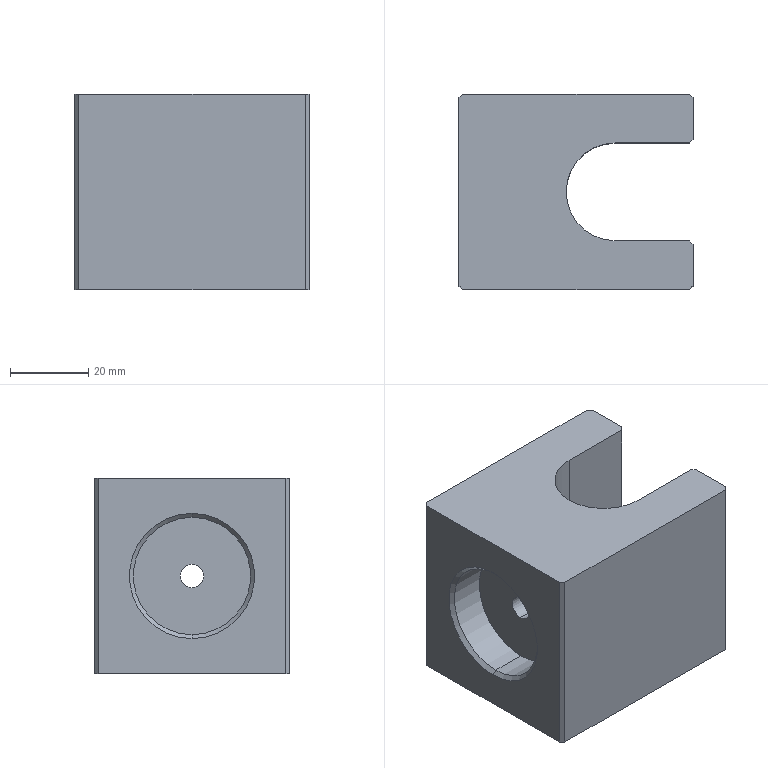Part | STEP file | Square block | 1 solid | 42 faces | box 60 x 50 x 50 mm | volume 104625 mm3 | plane 22 | cylinder 18 | cone 2 | commonest cylinder face diameters 3 x12 6 x2 25 x2 30 x2
STEP:
#1=CARTESIAN_POINT('',(-2.608,-19.158,50.));
#2=VERTEX_POINT('',#1);
#3=CARTESIAN_POINT('',(9.892,-6.658,50.));
#4=VERTEX_POINT('',#3);
#5=CARTESIAN_POINT('',(9.892,-19.158,50.));
#6=DIRECTION('',(0.,0.,-1.));
#7=DIRECTION('',(-1.,0.,0.));
#8=AXIS2_PLACEMENT_3D('',#5,#6,#7);
#9=CIRCLE('',#8,12.5);
#10=EDGE_CURVE('',#2,#4,#9,.T.);
#11=ORIENTED_EDGE('',*,*,#10,.F.);
#12=CARTESIAN_POINT('',(-2.608,-19.158,28.));
#13=VERTEX_POINT('',#12);
#14=CARTESIAN_POINT('',(-2.608,-19.158,50.));
#15=DIRECTION('',(0.,0.,-1.));
#16=VECTOR('',#15,1000.);
#17=LINE('',#14,#16);
#18=EDGE_CURVE('',#2,#13,#17,.T.);
#19=ORIENTED_EDGE('',*,*,#18,.T.);
#20=CARTESIAN_POINT('',(-2.608,-19.158,22.));
#21=VERTEX_POINT('',#20);
#22=CARTESIAN_POINT('',(-2.608,-19.158,22.));
#23=CARTESIAN_POINT('',(-2.608,-18.959,22.));
#24=CARTESIAN_POINT('',(-2.603,-18.764,22.02));
#25=CARTESIAN_POINT('',(-2.585,-18.379,22.096));
#26=CARTESIAN_POINT('',(-2.571,-18.188,22.154));
#27=CARTESIAN_POINT('',(-2.538,-17.825,22.305));
#28=CARTESIAN_POINT('',(-2.518,-17.653,22.397));
#29=CARTESIAN_POINT('',(-2.474,-17.328,22.615));
#30=CARTESIAN_POINT('',(-2.45,-17.174,22.741));
#31=CARTESIAN_POINT('',(-2.403,-16.899,23.017));
#32=CARTESIAN_POINT('',(-2.379,-16.775,23.167));
#33=CARTESIAN_POINT('',(-2.334,-16.556,23.495));
#34=CARTESIAN_POINT('',(-2.314,-16.463,23.668));
#35=CARTESIAN_POINT('',(-2.28,-16.313,24.029));
#36=CARTESIAN_POINT('',(-2.266,-16.255,24.218));
#37=CARTESIAN_POINT('',(-2.247,-16.177,24.606));
#38=CARTESIAN_POINT('',(-2.242,-16.158,24.801));
#39=CARTESIAN_POINT('',(-2.242,-16.158,25.194));
#40=CARTESIAN_POINT('',(-2.247,-16.177,25.393));
#41=CARTESIAN_POINT('',(-2.266,-16.254,25.779));
#42=CARTESIAN_POINT('',(-2.279,-16.311,25.966));
#43=CARTESIAN_POINT('',(-2.314,-16.462,26.33));
#44=CARTESIAN_POINT('',(-2.334,-16.555,26.505));
#45=CARTESIAN_POINT('',(-2.378,-16.772,26.829));
#46=CARTESIAN_POINT('',(-2.402,-16.897,26.981));
#47=CARTESIAN_POINT('',(-2.45,-17.175,27.259));
#48=CARTESIAN_POINT('',(-2.474,-17.325,27.383));
#49=CARTESIAN_POINT('',(-2.517,-17.649,27.6));
#50=CARTESIAN_POINT('',(-2.538,-17.825,27.695));
#51=CARTESIAN_POINT('',(-2.571,-18.187,27.845));
#52=CARTESIAN_POINT('',(-2.585,-18.374,27.902));
#53=CARTESIAN_POINT('',(-2.603,-18.76,27.98));
#54=CARTESIAN_POINT('',(-2.608,-18.959,28.));
#55=CARTESIAN_POINT('',(-2.608,-19.158,28.));
#56=B_SPLINE_CURVE_WITH_KNOTS('',3,(#22,#23,#24,#25,#26,#27,#28,#29,#30,#31,#32,#33,#34,#35,#36,#37,#38,#39,#40,#41,#42,#43,#44,#45,#46,#47,#48,#49,#50,#51,#52,#53,#54,#55),.UNSPECIFIED.,.F.,.F.,(4,2,2,2,2,2,2,2,2,2,2,2,2,2,2,2,4),(0.,0.0005882,0.001176,0.001765,0.002353,0.002941,0.003529,0.004117,0.004706,0.005294,0.005882,0.00647,0.007058,0.007646,0.008235,0.008823,0.009411),.UNSPECIFIED.);
#57=EDGE_CURVE('',#21,#13,#56,.T.);
#58=ORIENTED_EDGE('',*,*,#57,.F.);
#59=CARTESIAN_POINT('',(-2.608,-19.158,0.));
#60=VERTEX_POINT('',#59);
#61=CARTESIAN_POINT('',(-2.608,-19.158,50.));
#62=DIRECTION('',(0.,0.,-1.));
#63=VECTOR('',#62,1000.);
#64=LINE('',#61,#63);
#65=EDGE_CURVE('',#21,#60,#64,.T.);
#66=ORIENTED_EDGE('',*,*,#65,.T.);
#67=CARTESIAN_POINT('',(9.892,-6.658,0.));
#68=VERTEX_POINT('',#67);
#69=CARTESIAN_POINT('',(9.892,-19.158,0.));
#70=DIRECTION('',(0.,0.,-1.));
#71=DIRECTION('',(-1.,0.,0.));
#72=AXIS2_PLACEMENT_3D('',#69,#70,#71);
#73=CIRCLE('',#72,12.5);
#74=EDGE_CURVE('',#60,#68,#73,.T.);
#75=ORIENTED_EDGE('',*,*,#74,.T.);
#76=CARTESIAN_POINT('',(9.892,-6.658,50.));
#77=DIRECTION('',(0.,0.,1.));
#78=VECTOR('',#77,1000.);
#79=LINE('',#76,#78);
#80=EDGE_CURVE('',#68,#4,#79,.T.);
#81=ORIENTED_EDGE('',*,*,#80,.T.);
#82=EDGE_LOOP('',(#11,#19,#58,#66,#75,#81));
#83=FACE_OUTER_BOUND('',#82,.T.);
#84=CARTESIAN_POINT('',(9.892,-19.158,50.));
#85=DIRECTION('',(0.,0.,-1.));
#86=DIRECTION('',(-1.,0.,0.));
#87=AXIS2_PLACEMENT_3D('',#84,#85,#86);
#88=CYLINDRICAL_SURFACE('',#87,12.5);
#89=ADVANCED_FACE('',(#83),#88,.F.);
#90=CARTESIAN_POINT('',(-25.108,-2.158,24.));
#91=VERTEX_POINT('',#90);
#92=CARTESIAN_POINT('',(-25.108,-2.158,27.));
#93=VERTEX_POINT('',#92);
#94=CARTESIAN_POINT('',(-25.108,-2.158,25.5));
#95=DIRECTION('',(0.,1.,0.));
#96=DIRECTION('',(0.,0.,1.));
#97=AXIS2_PLACEMENT_3D('',#94,#95,#96);
#98=CIRCLE('',#97,1.5);
#99=EDGE_CURVE('',#91,#93,#98,.T.);
#100=ORIENTED_EDGE('',*,*,#99,.F.);
#101=CARTESIAN_POINT('',(-25.108,5.842,24.));
#102=VERTEX_POINT('',#101);
#103=CARTESIAN_POINT('',(-25.108,-2.158,24.));
#104=DIRECTION('',(0.,1.,0.));
#105=VECTOR('',#104,1000.);
#106=LINE('',#103,#105);
#107=EDGE_CURVE('',#91,#102,#106,.T.);
#108=ORIENTED_EDGE('',*,*,#107,.T.);
#109=CARTESIAN_POINT('',(-25.108,5.842,27.));
#110=VERTEX_POINT('',#109);
#111=CARTESIAN_POINT('',(-25.108,5.842,25.5));
#112=DIRECTION('',(0.,1.,0.));
#113=DIRECTION('',(0.,0.,1.));
#114=AXIS2_PLACEMENT_3D('',#111,#112,#113);
#115=CIRCLE('',#114,1.5);
#116=EDGE_CURVE('',#102,#110,#115,.T.);
#117=ORIENTED_EDGE('',*,*,#116,.T.);
#118=CARTESIAN_POINT('',(-25.108,-2.158,27.));
#119=DIRECTION('',(0.,1.,0.));
#120=VECTOR('',#119,1000.);
#121=LINE('',#118,#120);
#122=EDGE_CURVE('',#93,#110,#121,.T.);
#123=ORIENTED_EDGE('',*,*,#122,.F.);
#124=EDGE_LOOP('',(#100,#108,#117,#123));
#125=FACE_OUTER_BOUND('',#124,.T.);
#126=CARTESIAN_POINT('',(-25.108,-2.158,25.5));
#127=DIRECTION('',(0.,1.,0.));
#128=DIRECTION('',(0.,0.,1.));
#129=AXIS2_PLACEMENT_3D('',#126,#127,#128);
#130=CYLINDRICAL_SURFACE('',#129,1.5);
#131=ADVANCED_FACE('',(#125),#130,.F.);
#132=CARTESIAN_POINT('',(-15.108,-2.158,24.));
#133=VERTEX_POINT('',#132);
#134=CARTESIAN_POINT('',(-15.108,-2.158,27.));
#135=VERTEX_POINT('',#134);
#136=CARTESIAN_POINT('',(-15.108,-2.158,25.5));
#137=DIRECTION('',(0.,1.,0.));
#138=DIRECTION('',(0.,0.,1.));
#139=AXIS2_PLACEMENT_3D('',#136,#137,#138);
#140=CIRCLE('',#139,1.5);
#141=EDGE_CURVE('',#133,#135,#140,.T.);
#142=ORIENTED_EDGE('',*,*,#141,.F.);
#143=CARTESIAN_POINT('',(-15.108,5.842,24.));
#144=VERTEX_POINT('',#143);
#145=CARTESIAN_POINT('',(-15.108,-2.158,24.));
#146=DIRECTION('',(0.,1.,0.));
#147=VECTOR('',#146,1000.);
#148=LINE('',#145,#147);
#149=EDGE_CURVE('',#133,#144,#148,.T.);
#150=ORIENTED_EDGE('',*,*,#149,.T.);
#151=CARTESIAN_POINT('',(-15.108,5.842,27.));
#152=VERTEX_POINT('',#151);
#153=CARTESIAN_POINT('',(-15.108,5.842,25.5));
#154=DIRECTION('',(0.,1.,0.));
#155=DIRECTION('',(0.,0.,1.));
#156=AXIS2_PLACEMENT_3D('',#153,#154,#155);
#157=CIRCLE('',#156,1.5);
#158=EDGE_CURVE('',#144,#152,#157,.T.);
#159=ORIENTED_EDGE('',*,*,#158,.T.);
#160=CARTESIAN_POINT('',(-15.108,-2.158,27.));
#161=DIRECTION('',(0.,1.,0.));
#162=VECTOR('',#161,1000.);
#163=LINE('',#160,#162);
#164=EDGE_CURVE('',#135,#152,#163,.T.);
#165=ORIENTED_EDGE('',*,*,#164,.F.);
#166=EDGE_LOOP('',(#142,#150,#159,#165));
#167=FACE_OUTER_BOUND('',#166,.T.);
#168=CARTESIAN_POINT('',(-15.108,-2.158,25.5));
#169=DIRECTION('',(0.,1.,0.));
#170=DIRECTION('',(0.,0.,1.));
#171=AXIS2_PLACEMENT_3D('',#168,#169,#170);
#172=CYLINDRICAL_SURFACE('',#171,1.5);
#173=ADVANCED_FACE('',(#167),#172,.F.);
#174=CARTESIAN_POINT('',(-25.108,-2.158,39.));
#175=VERTEX_POINT('',#174);
#176=CARTESIAN_POINT('',(-25.108,-2.158,42.));
#177=VERTEX_POINT('',#176);
#178=CARTESIAN_POINT('',(-25.108,-2.158,40.5));
#179=DIRECTION('',(0.,1.,0.));
#180=DIRECTION('',(0.,0.,1.));
#181=AXIS2_PLACEMENT_3D('',#178,#179,#180);
#182=CIRCLE('',#181,1.5);
#183=EDGE_CURVE('',#175,#177,#182,.T.);
#184=ORIENTED_EDGE('',*,*,#183,.F.);
#185=CARTESIAN_POINT('',(-25.108,5.842,39.));
#186=VERTEX_POINT('',#185);
#187=CARTESIAN_POINT('',(-25.108,-2.158,39.));
#188=DIRECTION('',(0.,1.,0.));
#189=VECTOR('',#188,1000.);
#190=LINE('',#187,#189);
#191=EDGE_CURVE('',#175,#186,#190,.T.);
#192=ORIENTED_EDGE('',*,*,#191,.T.);
#193=CARTESIAN_POINT('',(-25.108,5.842,42.));
#194=VERTEX_POINT('',#193);
#195=CARTESIAN_POINT('',(-25.108,5.842,40.5));
#196=DIRECTION('',(0.,1.,0.));
#197=DIRECTION('',(0.,0.,1.));
#198=AXIS2_PLACEMENT_3D('',#195,#196,#197);
#199=CIRCLE('',#198,1.5);
#200=EDGE_CURVE('',#186,#194,#199,.T.);
#201=ORIENTED_EDGE('',*,*,#200,.T.);
#202=CARTESIAN_POINT('',(-25.108,-2.158,42.));
#203=DIRECTION('',(0.,1.,0.));
#204=VECTOR('',#203,1000.);
#205=LINE('',#202,#204);
#206=EDGE_CURVE('',#177,#194,#205,.T.);
#207=ORIENTED_EDGE('',*,*,#206,.F.);
#208=EDGE_LOOP('',(#184,#192,#201,#207));
#209=FACE_OUTER_BOUND('',#208,.T.);
#210=CARTESIAN_POINT('',(-25.108,-2.158,40.5));
#211=DIRECTION('',(0.,1.,0.));
#212=DIRECTION('',(0.,0.,1.));
#213=AXIS2_PLACEMENT_3D('',#210,#211,#212);
#214=CYLINDRICAL_SURFACE('',#213,1.5);
#215=ADVANCED_FACE('',(#209),#214,.F.);
#216=CARTESIAN_POINT('',(-15.108,-2.158,39.));
#217=VERTEX_POINT('',#216);
#218=CARTESIAN_POINT('',(-15.108,-2.158,42.));
#219=VERTEX_POINT('',#218);
#220=CARTESIAN_POINT('',(-15.108,-2.158,40.5));
#221=DIRECTION('',(0.,1.,0.));
#222=DIRECTION('',(0.,0.,1.));
#223=AXIS2_PLACEMENT_3D('',#220,#221,#222);
#224=CIRCLE('',#223,1.5);
#225=EDGE_CURVE('',#217,#219,#224,.T.);
#226=ORIENTED_EDGE('',*,*,#225,.F.);
#227=CARTESIAN_POINT('',(-15.108,5.842,39.));
#228=VERTEX_POINT('',#227);
#229=CARTESIAN_POINT('',(-15.108,-2.158,39.));
#230=DIRECTION('',(0.,1.,0.));
#231=VECTOR('',#230,1000.);
#232=LINE('',#229,#231);
#233=EDGE_CURVE('',#217,#228,#232,.T.);
#234=ORIENTED_EDGE('',*,*,#233,.T.);
#235=CARTESIAN_POINT('',(-15.108,5.842,42.));
#236=VERTEX_POINT('',#235);
#237=CARTESIAN_POINT('',(-15.108,5.842,40.5));
#238=DIRECTION('',(0.,1.,0.));
#239=DIRECTION('',(0.,0.,1.));
#240=AXIS2_PLACEMENT_3D('',#237,#238,#239);
#241=CIRCLE('',#240,1.5);
#242=EDGE_CURVE('',#228,#236,#241,.T.);
#243=ORIENTED_EDGE('',*,*,#242,.T.);
#244=CARTESIAN_POINT('',(-15.108,-2.158,42.));
#245=DIRECTION('',(0.,1.,0.));
#246=VECTOR('',#245,1000.);
#247=LINE('',#244,#246);
#248=EDGE_CURVE('',#219,#236,#247,.T.);
#249=ORIENTED_EDGE('',*,*,#248,.F.);
#250=EDGE_LOOP('',(#226,#234,#243,#249));
#251=FACE_OUTER_BOUND('',#250,.T.);
#252=CARTESIAN_POINT('',(-15.108,-2.158,40.5));
#253=DIRECTION('',(0.,1.,0.));
#254=DIRECTION('',(0.,0.,1.));
#255=AXIS2_PLACEMENT_3D('',#252,#253,#254);
#256=CYLINDRICAL_SURFACE('',#255,1.5);
#257=ADVANCED_FACE('',(#251),#256,.F.);
#258=CARTESIAN_POINT('',(-15.108,-2.158,9.));
#259=VERTEX_POINT('',#258);
#260=CARTESIAN_POINT('',(-15.108,-2.158,12.));
#261=VERTEX_POINT('',#260);
#262=CARTESIAN_POINT('',(-15.108,-2.158,10.5));
#263=DIRECTION('',(0.,1.,0.));
#264=DIRECTION('',(0.,0.,1.));
#265=AXIS2_PLACEMENT_3D('',#262,#263,#264);
#266=CIRCLE('',#265,1.5);
#267=EDGE_CURVE('',#259,#261,#266,.T.);
#268=ORIENTED_EDGE('',*,*,#267,.F.);
#269=CARTESIAN_POINT('',(-15.108,5.842,9.));
#270=VERTEX_POINT('',#269);
#271=CARTESIAN_POINT('',(-15.108,-2.158,9.));
#272=DIRECTION('',(0.,1.,0.));
#273=VECTOR('',#272,1000.);
#274=LINE('',#271,#273);
#275=EDGE_CURVE('',#259,#270,#274,.T.);
#276=ORIENTED_EDGE('',*,*,#275,.T.);
#277=CARTESIAN_POINT('',(-15.108,5.842,12.));
#278=VERTEX_POINT('',#277);
#279=CARTESIAN_POINT('',(-15.108,5.842,10.5));
#280=DIRECTION('',(0.,1.,0.));
#281=DIRECTION('',(0.,0.,1.));
#282=AXIS2_PLACEMENT_3D('',#279,#280,#281);
#283=CIRCLE('',#282,1.5);
#284=EDGE_CURVE('',#270,#278,#283,.T.);
#285=ORIENTED_EDGE('',*,*,#284,.T.);
#286=CARTESIAN_POINT('',(-15.108,-2.158,12.));
#287=DIRECTION('',(0.,1.,0.));
#288=VECTOR('',#287,1000.);
#289=LINE('',#286,#288);
#290=EDGE_CURVE('',#261,#278,#289,.T.);
#291=ORIENTED_EDGE('',*,*,#290,.F.);
#292=EDGE_LOOP('',(#268,#276,#285,#291));
#293=FACE_OUTER_BOUND('',#292,.T.);
#294=CARTESIAN_POINT('',(-15.108,-2.158,10.5));
#295=DIRECTION('',(0.,1.,0.));
#296=DIRECTION('',(0.,0.,1.));
#297=AXIS2_PLACEMENT_3D('',#294,#295,#296);
#298=CYLINDRICAL_SURFACE('',#297,1.5);
#299=ADVANCED_FACE('',(#293),#298,.F.);
#300=CARTESIAN_POINT('',(-25.108,-2.158,9.));
#301=VERTEX_POINT('',#300);
#302=CARTESIAN_POINT('',(-25.108,-2.158,12.));
#303=VERTEX_POINT('',#302);
#304=CARTESIAN_POINT('',(-25.108,-2.158,10.5));
#305=DIRECTION('',(0.,1.,0.));
#306=DIRECTION('',(0.,0.,1.));
#307=AXIS2_PLACEMENT_3D('',#304,#305,#306);
#308=CIRCLE('',#307,1.5);
#309=EDGE_CURVE('',#301,#303,#308,.T.);
#310=ORIENTED_EDGE('',*,*,#309,.F.);
#311=CARTESIAN_POINT('',(-25.108,5.842,9.));
#312=VERTEX_POINT('',#311);
#313=CARTESIAN_POINT('',(-25.108,-2.158,9.));
#314=DIRECTION('',(0.,1.,0.));
#315=VECTOR('',#314,1000.);
#316=LINE('',#313,#315);
#317=EDGE_CURVE('',#301,#312,#316,.T.);
#318=ORIENTED_EDGE('',*,*,#317,.T.);
#319=CARTESIAN_POINT('',(-25.108,5.842,12.));
#320=VERTEX_POINT('',#319);
#321=CARTESIAN_POINT('',(-25.108,5.842,10.5));
#322=DIRECTION('',(0.,1.,0.));
#323=DIRECTION('',(0.,0.,1.));
#324=AXIS2_PLACEMENT_3D('',#321,#322,#323);
#325=CIRCLE('',#324,1.5);
#326=EDGE_CURVE('',#312,#320,#325,.T.);
#327=ORIENTED_EDGE('',*,*,#326,.T.);
#328=CARTESIAN_POINT('',(-25.108,-2.158,12.));
#329=DIRECTION('',(0.,1.,0.));
#330=VECTOR('',#329,1000.);
#331=LINE('',#328,#330);
#332=EDGE_CURVE('',#303,#320,#331,.T.);
#333=ORIENTED_EDGE('',*,*,#332,.F.);
#334=EDGE_LOOP('',(#310,#318,#327,#333));
#335=FACE_OUTER_BOUND('',#334,.T.);
#336=CARTESIAN_POINT('',(-25.108,-2.158,10.5));
#337=DIRECTION('',(0.,1.,0.));
#338=DIRECTION('',(0.,0.,1.));
#339=AXIS2_PLACEMENT_3D('',#336,#337,#338);
#340=CYLINDRICAL_SURFACE('',#339,1.5);
#341=ADVANCED_FACE('',(#335),#340,.F.);
#342=CARTESIAN_POINT('',(-2.608,-19.158,28.));
#343=CARTESIAN_POINT('',(-2.608,-19.357,28.));
#344=CARTESIAN_POINT('',(-2.603,-19.552,27.98));
#345=CARTESIAN_POINT('',(-2.585,-19.937,27.904));
#346=CARTESIAN_POINT('',(-2.571,-20.128,27.846));
#347=CARTESIAN_POINT('',(-2.538,-20.491,27.695));
#348=CARTESIAN_POINT('',(-2.518,-20.663,27.603));
#349=CARTESIAN_POINT('',(-2.474,-20.988,27.385));
#350=CARTESIAN_POINT('',(-2.45,-21.142,27.259));
#351=CARTESIAN_POINT('',(-2.403,-21.417,26.983));
#352=CARTESIAN_POINT('',(-2.379,-21.541,26.833));
#353=CARTESIAN_POINT('',(-2.334,-21.761,26.505));
#354=CARTESIAN_POINT('',(-2.314,-21.853,26.332));
#355=CARTESIAN_POINT('',(-2.28,-22.003,25.971));
#356=CARTESIAN_POINT('',(-2.266,-22.061,25.782));
#357=CARTESIAN_POINT('',(-2.247,-22.139,25.394));
#358=CARTESIAN_POINT('',(-2.242,-22.158,25.199));
#359=CARTESIAN_POINT('',(-2.242,-22.158,24.806));
#360=CARTESIAN_POINT('',(-2.247,-22.139,24.607));
#361=CARTESIAN_POINT('',(-2.266,-22.062,24.221));
#362=CARTESIAN_POINT('',(-2.279,-22.005,24.034));
#363=CARTESIAN_POINT('',(-2.314,-21.854,23.67));
#364=CARTESIAN_POINT('',(-2.334,-21.761,23.495));
#365=CARTESIAN_POINT('',(-2.378,-21.544,23.171));
#366=CARTESIAN_POINT('',(-2.402,-21.419,23.019));
#367=CARTESIAN_POINT('',(-2.45,-21.141,22.741));
#368=CARTESIAN_POINT('',(-2.474,-20.991,22.617));
#369=CARTESIAN_POINT('',(-2.517,-20.667,22.4));
#370=CARTESIAN_POINT('',(-2.538,-20.491,22.305));
#371=CARTESIAN_POINT('',(-2.571,-20.129,22.155));
#372=CARTESIAN_POINT('',(-2.585,-19.942,22.098));
#373=CARTESIAN_POINT('',(-2.603,-19.556,22.02));
#374=CARTESIAN_POINT('',(-2.608,-19.357,22.));
#375=CARTESIAN_POINT('',(-2.608,-19.158,22.));
#376=B_SPLINE_CURVE_WITH_KNOTS('',3,(#342,#343,#344,#345,#346,#347,#348,#349,#350,#351,#352,#353,#354,#355,#356,#357,#358,#359,#360,#361,#362,#363,#364,#365,#366,#367,#368,#369,#370,#371,#372,#373,#374,#375),.UNSPECIFIED.,.F.,.F.,(4,2,2,2,2,2,2,2,2,2,2,2,2,2,2,2,4),(0.009411,0.009999,0.01059,0.01118,0.01176,0.01235,0.01294,0.01353,0.01412,0.0147,0.01529,0.01588,0.01647,0.01706,0.01765,0.01823,0.01882),.UNSPECIFIED.);
#377=EDGE_CURVE('',#13,#21,#376,.T.);
#378=ORIENTED_EDGE('',*,*,#377,.T.);
#379=CARTESIAN_POINT('',(-20.108,-19.158,22.));
#380=VERTEX_POINT('',#379);
#381=CARTESIAN_POINT('',(29.892,-19.158,22.));
#382=DIRECTION('',(-1.,0.,0.));
#383=VECTOR('',#382,1000.);
#384=LINE('',#381,#383);
#385=EDGE_CURVE('',#21,#380,#384,.T.);
#386=ORIENTED_EDGE('',*,*,#385,.T.);
#387=CARTESIAN_POINT('',(-20.108,-19.158,28.));
#388=VERTEX_POINT('',#387);
#389=CARTESIAN_POINT('',(-20.108,-19.158,25.));
#390=DIRECTION('',(1.,0.,0.));
#391=DIRECTION('',(0.,0.,1.));
#392=AXIS2_PLACEMENT_3D('',#389,#390,#391);
#393=CIRCLE('',#392,3.);
#394=EDGE_CURVE('',#388,#380,#393,.T.);
#395=ORIENTED_EDGE('',*,*,#394,.F.);
#396=CARTESIAN_POINT('',(29.892,-19.158,28.));
#397=DIRECTION('',(-1.,0.,0.));
#398=VECTOR('',#397,1000.);
#399=LINE('',#396,#398);
#400=EDGE_CURVE('',#13,#388,#399,.T.);
#401=ORIENTED_EDGE('',*,*,#400,.F.);
#402=EDGE_LOOP('',(#378,#386,#395,#401));
#403=FACE_OUTER_BOUND('',#402,.T.);
#404=CARTESIAN_POINT('',(29.892,-19.158,25.));
#405=DIRECTION('',(-1.,0.,0.));
#406=DIRECTION('',(0.,0.,1.));
#407=AXIS2_PLACEMENT_3D('',#404,#405,#406);
#408=CYLINDRICAL_SURFACE('',#407,3.);
#409=ADVANCED_FACE('',(#403),#408,.F.);
#410=CARTESIAN_POINT('',(-29.108,-19.158,10.));
#411=VERTEX_POINT('',#410);
#412=CARTESIAN_POINT('',(-29.108,-19.158,40.));
#413=VERTEX_POINT('',#412);
#414=CARTESIAN_POINT('',(-29.108,-19.158,25.));
#415=DIRECTION('',(-1.,0.,0.));
#416=DIRECTION('',(0.,0.,1.));
#417=AXIS2_PLACEMENT_3D('',#414,#415,#416);
#418=CIRCLE('',#417,15.);
#419=EDGE_CURVE('',#411,#413,#418,.T.);
#420=ORIENTED_EDGE('',*,*,#419,.F.);
#421=CARTESIAN_POINT('',(-30.108,-19.158,9.));
#422=VERTEX_POINT('',#421);
#423=CARTESIAN_POINT('',(-30.108,-19.158,9.));
#424=DIRECTION('',(-0.7071,0.,-0.7071));
#425=VECTOR('',#424,1000.);
#426=LINE('',#423,#425);
#427=EDGE_CURVE('',#411,#422,#426,.T.);
#428=ORIENTED_EDGE('',*,*,#427,.T.);
#429=CARTESIAN_POINT('',(-30.108,-19.158,41.));
#430=VERTEX_POINT('',#429);
#431=CARTESIAN_POINT('',(-30.108,-19.158,25.));
#432=DIRECTION('',(-1.,0.,0.));
#433=DIRECTION('',(0.,0.,1.));
#434=AXIS2_PLACEMENT_3D('',#431,#432,#433);
#435=CIRCLE('',#434,16.);
#436=EDGE_CURVE('',#422,#430,#435,.T.);
#437=ORIENTED_EDGE('',*,*,#436,.T.);
#438=CARTESIAN_POINT('',(-30.108,-19.158,41.));
#439=DIRECTION('',(-0.7071,0.,0.7071));
#440=VECTOR('',#439,1000.);
#441=LINE('',#438,#440);
#442=EDGE_CURVE('',#413,#430,#441,.T.);
#443=ORIENTED_EDGE('',*,*,#442,.F.);
#444=EDGE_LOOP('',(#420,#428,#437,#443));
#445=FACE_OUTER_BOUND('',#444,.T.);
#446=CARTESIAN_POINT('',(-30.108,-19.158,25.));
#447=DIRECTION('',(-1.,0.,0.));
#448=DIRECTION('',(0.,0.,1.));
#449=AXIS2_PLACEMENT_3D('',#446,#447,#448);
#450=CONICAL_SURFACE('',#449,16.,0.7854);
#451=ADVANCED_FACE('',(#445),#450,.F.);
#452=CARTESIAN_POINT('',(-20.108,-19.158,10.));
#453=VERTEX_POINT('',#452);
#454=CARTESIAN_POINT('',(-20.108,-19.158,40.));
#455=VERTEX_POINT('',#454);
#456=CARTESIAN_POINT('',(-20.108,-19.158,25.));
#457=DIRECTION('',(-1.,0.,0.));
#458=DIRECTION('',(0.,0.,1.));
#459=AXIS2_PLACEMENT_3D('',#456,#457,#458);
#460=CIRCLE('',#459,15.);
#461=EDGE_CURVE('',#453,#455,#460,.T.);
#462=ORIENTED_EDGE('',*,*,#461,.F.);
#463=CARTESIAN_POINT('',(-20.108,-19.158,10.));
#464=DIRECTION('',(-1.,0.,0.));
#465=VECTOR('',#464,1000.);
#466=LINE('',#463,#465);
#467=EDGE_CURVE('',#453,#411,#466,.T.);
#468=ORIENTED_EDGE('',*,*,#467,.T.);
#469=ORIENTED_EDGE('',*,*,#419,.T.);
#470=CARTESIAN_POINT('',(-20.108,-19.158,40.));
#471=DIRECTION('',(-1.,0.,0.));
#472=VECTOR('',#471,1000.);
#473=LINE('',#470,#472);
#474=EDGE_CURVE('',#455,#413,#473,.T.);
#475=ORIENTED_EDGE('',*,*,#474,.F.);
#476=EDGE_LOOP('',(#462,#468,#469,#475));
#477=FACE_OUTER_BOUND('',#476,.T.);
#478=CARTESIAN_POINT('',(-20.108,-19.158,25.));
#479=DIRECTION('',(-1.,0.,0.));
#480=DIRECTION('',(0.,0.,1.));
#481=AXIS2_PLACEMENT_3D('',#478,#479,#480);
#482=CYLINDRICAL_SURFACE('',#481,15.);
#483=ADVANCED_FACE('',(#477),#482,.F.);
#484=CARTESIAN_POINT('',(-29.108,-44.158,0.));
#485=VERTEX_POINT('',#484);
#486=CARTESIAN_POINT('',(-29.108,-44.158,50.));
#487=VERTEX_POINT('',#486);
#488=CARTESIAN_POINT('',(-29.108,-44.158,50.));
#489=DIRECTION('',(0.,0.,1.));
#490=VECTOR('',#489,1000.);
#491=LINE('',#488,#490);
#492=EDGE_CURVE('',#485,#487,#491,.T.);
#493=ORIENTED_EDGE('',*,*,#492,.F.);
#494=CARTESIAN_POINT('',(28.892,-44.158,0.));
#495=VERTEX_POINT('',#494);
#496=CARTESIAN_POINT('',(-30.108,-44.158,0.));
#497=DIRECTION('',(-1.,0.,0.));
#498=VECTOR('',#497,1000.);
#499=LINE('',#496,#498);
#500=EDGE_CURVE('',#495,#485,#499,.T.);
#501=ORIENTED_EDGE('',*,*,#500,.F.);
#502=CARTESIAN_POINT('',(28.892,-44.158,50.));
#503=VERTEX_POINT('',#502);
#504=CARTESIAN_POINT('',(28.892,-44.158,50.));
#505=DIRECTION('',(0.,0.,-1.));
#506=VECTOR('',#505,1000.);
#507=LINE('',#504,#506);
#508=EDGE_CURVE('',#503,#495,#507,.T.);
#509=ORIENTED_EDGE('',*,*,#508,.F.);
#510=CARTESIAN_POINT('',(-30.108,-44.158,50.));
#511=DIRECTION('',(1.,0.,0.));
#512=VECTOR('',#511,1000.);
#513=LINE('',#510,#512);
#514=EDGE_CURVE('',#487,#503,#513,.T.);
#515=ORIENTED_EDGE('',*,*,#514,.F.);
#516=EDGE_LOOP('',(#493,#501,#509,#515));
#517=FACE_OUTER_BOUND('',#516,.T.);
#518=CARTESIAN_POINT('',(-30.108,-44.158,50.));
#519=DIRECTION('',(0.,1.,0.));
#520=DIRECTION('',(0.,0.,1.));
#521=AXIS2_PLACEMENT_3D('',#518,#519,#520);
#522=PLANE('',#521);
#523=ADVANCED_FACE('',(#517),#522,.F.);
#524=CARTESIAN_POINT('',(28.892,5.842,50.));
#525=VERTEX_POINT('',#524);
#526=CARTESIAN_POINT('',(-29.108,5.842,50.));
#527=VERTEX_POINT('',#526);
#528=CARTESIAN_POINT('',(9.892,5.842,50.));
#529=DIRECTION('',(-1.,0.,0.));
#530=VECTOR('',#529,1000.);
#531=LINE('',#528,#530);
#532=EDGE_CURVE('',#525,#527,#531,.T.);
#533=ORIENTED_EDGE('',*,*,#532,.T.);
#534=CARTESIAN_POINT('',(-30.108,4.842,50.));
#535=VERTEX_POINT('',#534);
#536=CARTESIAN_POINT('',(-30.108,4.842,50.));
#537=DIRECTION('',(-0.7071,-0.7071,0.));
#538=VECTOR('',#537,1000.);
#539=LINE('',#536,#538);
#540=EDGE_CURVE('',#527,#535,#539,.T.);
#541=ORIENTED_EDGE('',*,*,#540,.T.);
#542=CARTESIAN_POINT('',(-30.108,-43.158,50.));
#543=VERTEX_POINT('',#542);
#544=CARTESIAN_POINT('',(-30.108,-19.158,50.));
#545=DIRECTION('',(0.,-1.,0.));
#546=VECTOR('',#545,1000.);
#547=LINE('',#544,#546);
#548=EDGE_CURVE('',#535,#543,#547,.T.);
#549=ORIENTED_EDGE('',*,*,#548,.T.);
#550=CARTESIAN_POINT('',(-30.108,-43.158,50.));
#551=DIRECTION('',(0.7071,-0.7071,0.));
#552=VECTOR('',#551,1000.);
#553=LINE('',#550,#552);
#554=EDGE_CURVE('',#543,#487,#553,.T.);
#555=ORIENTED_EDGE('',*,*,#554,.T.);
#556=ORIENTED_EDGE('',*,*,#514,.T.);
#557=CARTESIAN_POINT('',(29.892,-43.158,50.));
#558=VERTEX_POINT('',#557);
#559=CARTESIAN_POINT('',(28.892,-44.158,50.));
#560=DIRECTION('',(0.7071,0.7071,0.));
#561=VECTOR('',#560,1000.);
#562=LINE('',#559,#561);
#563=EDGE_CURVE('',#503,#558,#562,.T.);
#564=ORIENTED_EDGE('',*,*,#563,.T.);
#565=CARTESIAN_POINT('',(29.892,-32.658,50.));
#566=VERTEX_POINT('',#565);
#567=CARTESIAN_POINT('',(29.892,-19.158,50.));
#568=DIRECTION('',(0.,1.,0.));
#569=VECTOR('',#568,1000.);
#570=LINE('',#567,#569);
#571=EDGE_CURVE('',#558,#566,#570,.T.);
#572=ORIENTED_EDGE('',*,*,#571,.T.);
#573=CARTESIAN_POINT('',(28.892,-31.658,50.));
#574=VERTEX_POINT('',#573);
#575=CARTESIAN_POINT('',(28.892,-31.658,50.));
#576=DIRECTION('',(-0.7071,0.7071,0.));
#577=VECTOR('',#576,1000.);
#578=LINE('',#575,#577);
#579=EDGE_CURVE('',#566,#574,#578,.T.);
#580=ORIENTED_EDGE('',*,*,#579,.T.);
#581=CARTESIAN_POINT('',(9.892,-31.658,50.));
#582=VERTEX_POINT('',#581);
#583=CARTESIAN_POINT('',(9.892,-31.658,50.));
#584=DIRECTION('',(-1.,0.,0.));
#585=VECTOR('',#584,1000.);
#586=LINE('',#583,#585);
#587=EDGE_CURVE('',#574,#582,#586,.T.);
#588=ORIENTED_EDGE('',*,*,#587,.T.);
#589=CARTESIAN_POINT('',(9.892,-19.158,50.));
#590=DIRECTION('',(0.,0.,-1.));
#591=DIRECTION('',(-1.,0.,0.));
#592=AXIS2_PLACEMENT_3D('',#589,#590,#591);
#593=CIRCLE('',#592,12.5);
#594=EDGE_CURVE('',#582,#2,#593,.T.);
#595=ORIENTED_EDGE('',*,*,#594,.T.);
#596=ORIENTED_EDGE('',*,*,#10,.T.);
#597=CARTESIAN_POINT('',(28.892,-6.658,50.));
#598=VERTEX_POINT('',#597);
#599=CARTESIAN_POINT('',(9.892,-6.658,50.));
#600=DIRECTION('',(1.,0.,0.));
#601=VECTOR('',#600,1000.);
#602=LINE('',#599,#601);
#603=EDGE_CURVE('',#4,#598,#602,.T.);
#604=ORIENTED_EDGE('',*,*,#603,.T.);
#605=CARTESIAN_POINT('',(29.892,-5.658,50.));
#606=VERTEX_POINT('',#605);
#607=CARTESIAN_POINT('',(29.892,-5.658,50.));
#608=DIRECTION('',(0.7071,0.7071,0.));
#609=VECTOR('',#608,1000.);
#610=LINE('',#607,#609);
#611=EDGE_CURVE('',#598,#606,#610,.T.);
#612=ORIENTED_EDGE('',*,*,#611,.T.);
#613=CARTESIAN_POINT('',(29.892,4.842,50.));
#614=VERTEX_POINT('',#613);
#615=CARTESIAN_POINT('',(29.892,-19.158,50.));
#616=DIRECTION('',(0.,1.,0.));
#617=VECTOR('',#616,1000.);
#618=LINE('',#615,#617);
#619=EDGE_CURVE('',#606,#614,#618,.T.);
#620=ORIENTED_EDGE('',*,*,#619,.T.);
#621=CARTESIAN_POINT('',(28.892,5.842,50.));
#622=DIRECTION('',(-0.7071,0.7071,0.));
#623=VECTOR('',#622,1000.);
#624=LINE('',#621,#623);
#625=EDGE_CURVE('',#614,#525,#624,.T.);
#626=ORIENTED_EDGE('',*,*,#625,.T.);
#627=EDGE_LOOP('',(#533,#541,#549,#555,#556,#564,#572,#580,#588,#595,#596,#604,#612,#620,#626));
#628=FACE_OUTER_BOUND('',#627,.T.);
#629=CARTESIAN_POINT('',(9.892,-19.158,50.));
#630=DIRECTION('',(0.,0.,1.));
#631=DIRECTION('',(1.,0.,0.));
#632=AXIS2_PLACEMENT_3D('',#629,#630,#631);
#633=PLANE('',#632);
#634=ADVANCED_FACE('',(#628),#633,.T.);
#635=CARTESIAN_POINT('',(-30.108,-43.158,0.));
#636=VERTEX_POINT('',#635);
#637=CARTESIAN_POINT('',(-30.108,-43.158,50.));
#638=DIRECTION('',(0.,0.,1.));
#639=VECTOR('',#638,1000.);
#640=LINE('',#637,#639);
#641=EDGE_CURVE('',#636,#543,#640,.T.);
#642=ORIENTED_EDGE('',*,*,#641,.F.);
#643=CARTESIAN_POINT('',(-29.108,-44.158,0.));
#644=DIRECTION('',(-0.7071,0.7071,0.));
#645=VECTOR('',#644,1000.);
#646=LINE('',#643,#645);
#647=EDGE_CURVE('',#485,#636,#646,.T.);
#648=ORIENTED_EDGE('',*,*,#647,.F.);
#649=ORIENTED_EDGE('',*,*,#492,.T.);
#650=ORIENTED_EDGE('',*,*,#554,.F.);
#651=EDGE_LOOP('',(#642,#648,#649,#650));
#652=FACE_OUTER_BOUND('',#651,.T.);
#653=CARTESIAN_POINT('',(-29.108,-44.158,50.));
#654=DIRECTION('',(0.7071,0.7071,0.));
#655=DIRECTION('',(-0.7071,0.7071,0.));
#656=AXIS2_PLACEMENT_3D('',#653,#654,#655);
#657=PLANE('',#656);
#658=ADVANCED_FACE('',(#652),#657,.F.);
#659=ORIENTED_EDGE('',*,*,#647,.T.);
#660=CARTESIAN_POINT('',(-30.108,4.842,0.));
#661=VERTEX_POINT('',#660);
#662=CARTESIAN_POINT('',(-30.108,-19.158,0.));
#663=DIRECTION('',(0.,-1.,0.));
#664=VECTOR('',#663,1000.);
#665=LINE('',#662,#664);
#666=EDGE_CURVE('',#661,#636,#665,.T.);
#667=ORIENTED_EDGE('',*,*,#666,.F.);
#668=CARTESIAN_POINT('',(-29.108,5.842,0.));
#669=VERTEX_POINT('',#668);
#670=CARTESIAN_POINT('',(-30.108,4.842,0.));
#671=DIRECTION('',(0.7071,0.7071,0.));
#672=VECTOR('',#671,1000.);
#673=LINE('',#670,#672);
#674=EDGE_CURVE('',#661,#669,#673,.T.);
#675=ORIENTED_EDGE('',*,*,#674,.T.);
#676=CARTESIAN_POINT('',(28.892,5.842,0.));
#677=VERTEX_POINT('',#676);
#678=CARTESIAN_POINT('',(9.892,5.842,0.));
#679=DIRECTION('',(-1.,0.,0.));
#680=VECTOR('',#679,1000.);
#681=LINE('',#678,#680);
#682=EDGE_CURVE('',#677,#669,#681,.T.);
#683=ORIENTED_EDGE('',*,*,#682,.F.);
#684=CARTESIAN_POINT('',(29.892,4.842,0.));
#685=VERTEX_POINT('',#684);
#686=CARTESIAN_POINT('',(28.892,5.842,0.));
#687=DIRECTION('',(0.7071,-0.7071,0.));
#688=VECTOR('',#687,1000.);
#689=LINE('',#686,#688);
#690=EDGE_CURVE('',#677,#685,#689,.T.);
#691=ORIENTED_EDGE('',*,*,#690,.T.);
#692=CARTESIAN_POINT('',(29.892,-5.658,0.));
#693=VERTEX_POINT('',#692);
#694=CARTESIAN_POINT('',(29.892,-19.158,0.));
#695=DIRECTION('',(0.,1.,0.));
#696=VECTOR('',#695,1000.);
#697=LINE('',#694,#696);
#698=EDGE_CURVE('',#693,#685,#697,.T.);
#699=ORIENTED_EDGE('',*,*,#698,.F.);
#700=CARTESIAN_POINT('',(28.892,-6.658,0.));
#701=VERTEX_POINT('',#700);
#702=CARTESIAN_POINT('',(29.892,-5.658,0.));
#703=DIRECTION('',(-0.7071,-0.7071,0.));
#704=VECTOR('',#703,1000.);
#705=LINE('',#702,#704);
#706=EDGE_CURVE('',#693,#701,#705,.T.);
#707=ORIENTED_EDGE('',*,*,#706,.T.);
#708=CARTESIAN_POINT('',(9.892,-6.658,0.));
#709=DIRECTION('',(1.,0.,0.));
#710=VECTOR('',#709,1000.);
#711=LINE('',#708,#710);
#712=EDGE_CURVE('',#68,#701,#711,.T.);
#713=ORIENTED_EDGE('',*,*,#712,.F.);
#714=ORIENTED_EDGE('',*,*,#74,.F.);
#715=CARTESIAN_POINT('',(9.892,-31.658,0.));
#716=VERTEX_POINT('',#715);
#717=CARTESIAN_POINT('',(9.892,-19.158,0.));
#718=DIRECTION('',(0.,0.,-1.));
#719=DIRECTION('',(-1.,0.,0.));
#720=AXIS2_PLACEMENT_3D('',#717,#718,#719);
#721=CIRCLE('',#720,12.5);
#722=EDGE_CURVE('',#716,#60,#721,.T.);
#723=ORIENTED_EDGE('',*,*,#722,.F.);
#724=CARTESIAN_POINT('',(28.892,-31.658,0.));
#725=VERTEX_POINT('',#724);
#726=CARTESIAN_POINT('',(9.892,-31.658,0.));
#727=DIRECTION('',(-1.,0.,0.));
#728=VECTOR('',#727,1000.);
#729=LINE('',#726,#728);
#730=EDGE_CURVE('',#725,#716,#729,.T.);
#731=ORIENTED_EDGE('',*,*,#730,.F.);
#732=CARTESIAN_POINT('',(29.892,-32.658,0.));
#733=VERTEX_POINT('',#732);
#734=CARTESIAN_POINT('',(28.892,-31.658,0.));
#735=DIRECTION('',(0.7071,-0.7071,0.));
#736=VECTOR('',#735,1000.);
#737=LINE('',#734,#736);
#738=EDGE_CURVE('',#725,#733,#737,.T.);
#739=ORIENTED_EDGE('',*,*,#738,.T.);
#740=CARTESIAN_POINT('',(29.892,-43.158,0.));
#741=VERTEX_POINT('',#740);
#742=CARTESIAN_POINT('',(29.892,-19.158,0.));
#743=DIRECTION('',(0.,1.,0.));
#744=VECTOR('',#743,1000.);
#745=LINE('',#742,#744);
#746=EDGE_CURVE('',#741,#733,#745,.T.);
#747=ORIENTED_EDGE('',*,*,#746,.F.);
#748=CARTESIAN_POINT('',(28.892,-44.158,0.));
#749=DIRECTION('',(0.7071,0.7071,0.));
#750=VECTOR('',#749,1000.);
#751=LINE('',#748,#750);
#752=EDGE_CURVE('',#495,#741,#751,.T.);
#753=ORIENTED_EDGE('',*,*,#752,.F.);
#754=ORIENTED_EDGE('',*,*,#500,.T.);
#755=EDGE_LOOP('',(#659,#667,#675,#683,#691,#699,#707,#713,#714,#723,#731,#739,#747,#753,#754));
#756=FACE_OUTER_BOUND('',#755,.T.);
#757=CARTESIAN_POINT('',(9.892,-19.158,0.));
#758=DIRECTION('',(0.,0.,1.));
#759=DIRECTION('',(1.,0.,0.));
#760=AXIS2_PLACEMENT_3D('',#757,#758,#759);
#761=PLANE('',#760);
#762=ADVANCED_FACE('',(#756),#761,.F.);
#763=ORIENTED_EDGE('',*,*,#508,.T.);
#764=ORIENTED_EDGE('',*,*,#752,.T.);
#765=CARTESIAN_POINT('',(29.892,-43.158,50.));
#766=DIRECTION('',(0.,0.,-1.));
#767=VECTOR('',#766,1000.);
#768=LINE('',#765,#767);
#769=EDGE_CURVE('',#558,#741,#768,.T.);
#770=ORIENTED_EDGE('',*,*,#769,.F.);
#771=ORIENTED_EDGE('',*,*,#563,.F.);
#772=EDGE_LOOP('',(#763,#764,#770,#771));
#773=FACE_OUTER_BOUND('',#772,.T.);
#774=CARTESIAN_POINT('',(29.892,-43.158,50.));
#775=DIRECTION('',(-0.7071,0.7071,0.));
#776=DIRECTION('',(-0.7071,-0.7071,0.));
#777=AXIS2_PLACEMENT_3D('',#774,#775,#776);
#778=PLANE('',#777);
#779=ADVANCED_FACE('',(#773),#778,.F.);
#780=CARTESIAN_POINT('',(-29.108,5.842,50.));
#781=DIRECTION('',(0.,0.,-1.));
#782=VECTOR('',#781,1000.);
#783=LINE('',#780,#782);
#784=EDGE_CURVE('',#527,#669,#783,.T.);
#785=ORIENTED_EDGE('',*,*,#784,.F.);
#786=ORIENTED_EDGE('',*,*,#532,.F.);
#787=CARTESIAN_POINT('',(28.892,5.842,50.));
#788=DIRECTION('',(0.,0.,1.));
#789=VECTOR('',#788,1000.);
#790=LINE('',#787,#789);
#791=EDGE_CURVE('',#677,#525,#790,.T.);
#792=ORIENTED_EDGE('',*,*,#791,.F.);
#793=ORIENTED_EDGE('',*,*,#682,.T.);
#794=EDGE_LOOP('',(#785,#786,#792,#793));
#795=FACE_OUTER_BOUND('',#794,.T.);
#796=CARTESIAN_POINT('',(-25.108,5.842,25.5));
#797=DIRECTION('',(0.,1.,0.));
#798=DIRECTION('',(0.,0.,1.));
#799=AXIS2_PLACEMENT_3D('',#796,#797,#798);
#800=CIRCLE('',#799,1.5);
#801=EDGE_CURVE('',#110,#102,#800,.T.);
#802=ORIENTED_EDGE('',*,*,#801,.F.);
#803=ORIENTED_EDGE('',*,*,#116,.F.);
#804=EDGE_LOOP('',(#802,#803));
#805=FACE_BOUND('',#804,.T.);
#806=CARTESIAN_POINT('',(-15.108,5.842,25.5));
#807=DIRECTION('',(0.,1.,0.));
#808=DIRECTION('',(0.,0.,1.));
#809=AXIS2_PLACEMENT_3D('',#806,#807,#808);
#810=CIRCLE('',#809,1.5);
#811=EDGE_CURVE('',#152,#144,#810,.T.);
#812=ORIENTED_EDGE('',*,*,#811,.F.);
#813=ORIENTED_EDGE('',*,*,#158,.F.);
#814=EDGE_LOOP('',(#812,#813));
#815=FACE_BOUND('',#814,.T.);
#816=CARTESIAN_POINT('',(-25.108,5.842,40.5));
#817=DIRECTION('',(0.,1.,0.));
#818=DIRECTION('',(0.,0.,1.));
#819=AXIS2_PLACEMENT_3D('',#816,#817,#818);
#820=CIRCLE('',#819,1.5);
#821=EDGE_CURVE('',#194,#186,#820,.T.);
#822=ORIENTED_EDGE('',*,*,#821,.F.);
#823=ORIENTED_EDGE('',*,*,#200,.F.);
#824=EDGE_LOOP('',(#822,#823));
#825=FACE_BOUND('',#824,.T.);
#826=CARTESIAN_POINT('',(-15.108,5.842,40.5));
#827=DIRECTION('',(0.,1.,0.));
#828=DIRECTION('',(0.,0.,1.));
#829=AXIS2_PLACEMENT_3D('',#826,#827,#828);
#830=CIRCLE('',#829,1.5);
#831=EDGE_CURVE('',#236,#228,#830,.T.);
#832=ORIENTED_EDGE('',*,*,#831,.F.);
#833=ORIENTED_EDGE('',*,*,#242,.F.);
#834=EDGE_LOOP('',(#832,#833));
#835=FACE_BOUND('',#834,.T.);
#836=CARTESIAN_POINT('',(-15.108,5.842,10.5));
#837=DIRECTION('',(0.,1.,0.));
#838=DIRECTION('',(0.,0.,1.));
#839=AXIS2_PLACEMENT_3D('',#836,#837,#838);
#840=CIRCLE('',#839,1.5);
#841=EDGE_CURVE('',#278,#270,#840,.T.);
#842=ORIENTED_EDGE('',*,*,#841,.F.);
#843=ORIENTED_EDGE('',*,*,#284,.F.);
#844=EDGE_LOOP('',(#842,#843));
#845=FACE_BOUND('',#844,.T.);
#846=CARTESIAN_POINT('',(-25.108,5.842,10.5));
#847=DIRECTION('',(0.,1.,0.));
#848=DIRECTION('',(0.,0.,1.));
#849=AXIS2_PLACEMENT_3D('',#846,#847,#848);
#850=CIRCLE('',#849,1.5);
#851=EDGE_CURVE('',#320,#312,#850,.T.);
#852=ORIENTED_EDGE('',*,*,#851,.F.);
#853=ORIENTED_EDGE('',*,*,#326,.F.);
#854=EDGE_LOOP('',(#852,#853));
#855=FACE_BOUND('',#854,.T.);
#856=CARTESIAN_POINT('',(-30.108,5.842,50.));
#857=DIRECTION('',(0.,-1.,0.));
#858=DIRECTION('',(0.,0.,-1.));
#859=AXIS2_PLACEMENT_3D('',#856,#857,#858);
#860=PLANE('',#859);
#861=ADVANCED_FACE('',(#795,#805,#815,#825,#835,#845,#855),#860,.F.);
#862=CARTESIAN_POINT('',(29.892,-5.658,50.));
#863=DIRECTION('',(0.,0.,1.));
#864=VECTOR('',#863,1000.);
#865=LINE('',#862,#864);
#866=EDGE_CURVE('',#693,#606,#865,.T.);
#867=ORIENTED_EDGE('',*,*,#866,.F.);
#868=ORIENTED_EDGE('',*,*,#698,.T.);
#869=CARTESIAN_POINT('',(29.892,4.842,50.));
#870=DIRECTION('',(0.,0.,-1.));
#871=VECTOR('',#870,1000.);
#872=LINE('',#869,#871);
#873=EDGE_CURVE('',#614,#685,#872,.T.);
#874=ORIENTED_EDGE('',*,*,#873,.F.);
#875=ORIENTED_EDGE('',*,*,#619,.F.);
#876=EDGE_LOOP('',(#867,#868,#874,#875));
#877=FACE_OUTER_BOUND('',#876,.T.);
#878=CARTESIAN_POINT('',(29.892,5.842,50.));
#879=DIRECTION('',(-1.,0.,0.));
#880=DIRECTION('',(0.,0.,1.));
#881=AXIS2_PLACEMENT_3D('',#878,#879,#880);
#882=PLANE('',#881);
#883=ADVANCED_FACE('',(#877),#882,.F.);
#884=CARTESIAN_POINT('',(28.892,-6.658,50.));
#885=DIRECTION('',(0.,0.,-1.));
#886=VECTOR('',#885,1000.);
#887=LINE('',#884,#886);
#888=EDGE_CURVE('',#598,#701,#887,.T.);
#889=ORIENTED_EDGE('',*,*,#888,.F.);
#890=ORIENTED_EDGE('',*,*,#603,.F.);
#891=ORIENTED_EDGE('',*,*,#80,.F.);
#892=ORIENTED_EDGE('',*,*,#712,.T.);
#893=EDGE_LOOP('',(#889,#890,#891,#892));
#894=FACE_OUTER_BOUND('',#893,.T.);
#895=CARTESIAN_POINT('',(29.892,-6.658,50.));
#896=DIRECTION('',(0.,1.,0.));
#897=DIRECTION('',(-1.,0.,0.));
#898=AXIS2_PLACEMENT_3D('',#895,#896,#897);
#899=PLANE('',#898);
#900=ADVANCED_FACE('',(#894),#899,.F.);
#901=ORIENTED_EDGE('',*,*,#18,.F.);
#902=ORIENTED_EDGE('',*,*,#594,.F.);
#903=CARTESIAN_POINT('',(9.892,-31.658,50.));
#904=DIRECTION('',(0.,0.,1.));
#905=VECTOR('',#904,1000.);
#906=LINE('',#903,#905);
#907=EDGE_CURVE('',#716,#582,#906,.T.);
#908=ORIENTED_EDGE('',*,*,#907,.F.);
#909=ORIENTED_EDGE('',*,*,#722,.T.);
#910=ORIENTED_EDGE('',*,*,#65,.F.);
#911=ORIENTED_EDGE('',*,*,#377,.F.);
#912=EDGE_LOOP('',(#901,#902,#908,#909,#910,#911));
#913=FACE_OUTER_BOUND('',#912,.T.);
#914=CARTESIAN_POINT('',(9.892,-19.158,50.));
#915=DIRECTION('',(0.,0.,-1.));
#916=DIRECTION('',(-1.,0.,0.));
#917=AXIS2_PLACEMENT_3D('',#914,#915,#916);
#918=CYLINDRICAL_SURFACE('',#917,12.5);
#919=ADVANCED_FACE('',(#913),#918,.F.);
#920=CARTESIAN_POINT('',(28.892,-31.658,50.));
#921=DIRECTION('',(0.,0.,1.));
#922=VECTOR('',#921,1000.);
#923=LINE('',#920,#922);
#924=EDGE_CURVE('',#725,#574,#923,.T.);
#925=ORIENTED_EDGE('',*,*,#924,.F.);
#926=ORIENTED_EDGE('',*,*,#730,.T.);
#927=ORIENTED_EDGE('',*,*,#907,.T.);
#928=ORIENTED_EDGE('',*,*,#587,.F.);
#929=EDGE_LOOP('',(#925,#926,#927,#928));
#930=FACE_OUTER_BOUND('',#929,.T.);
#931=CARTESIAN_POINT('',(9.892,-31.658,50.));
#932=DIRECTION('',(0.,-1.,0.));
#933=DIRECTION('',(0.,0.,-1.));
#934=AXIS2_PLACEMENT_3D('',#931,#932,#933);
#935=PLANE('',#934);
#936=ADVANCED_FACE('',(#930),#935,.F.);
#937=ORIENTED_EDGE('',*,*,#769,.T.);
#938=ORIENTED_EDGE('',*,*,#746,.T.);
#939=CARTESIAN_POINT('',(29.892,-32.658,50.));
#940=DIRECTION('',(0.,0.,-1.));
#941=VECTOR('',#940,1000.);
#942=LINE('',#939,#941);
#943=EDGE_CURVE('',#566,#733,#942,.T.);
#944=ORIENTED_EDGE('',*,*,#943,.F.);
#945=ORIENTED_EDGE('',*,*,#571,.F.);
#946=EDGE_LOOP('',(#937,#938,#944,#945));
#947=FACE_OUTER_BOUND('',#946,.T.);
#948=CARTESIAN_POINT('',(29.892,-31.658,50.));
#949=DIRECTION('',(-1.,0.,0.));
#950=DIRECTION('',(0.,-1.,0.));
#951=AXIS2_PLACEMENT_3D('',#948,#949,#950);
#952=PLANE('',#951);
#953=ADVANCED_FACE('',(#947),#952,.F.);
#954=ORIENTED_EDGE('',*,*,#641,.T.);
#955=ORIENTED_EDGE('',*,*,#548,.F.);
#956=CARTESIAN_POINT('',(-30.108,4.842,50.));
#957=DIRECTION('',(0.,0.,1.));
#958=VECTOR('',#957,1000.);
#959=LINE('',#956,#958);
#960=EDGE_CURVE('',#661,#535,#959,.T.);
#961=ORIENTED_EDGE('',*,*,#960,.F.);
#962=ORIENTED_EDGE('',*,*,#666,.T.);
#963=EDGE_LOOP('',(#954,#955,#961,#962));
#964=FACE_OUTER_BOUND('',#963,.T.);
#965=CARTESIAN_POINT('',(-30.108,-19.158,25.));
#966=DIRECTION('',(-1.,0.,0.));
#967=DIRECTION('',(0.,0.,1.));
#968=AXIS2_PLACEMENT_3D('',#965,#966,#967);
#969=CIRCLE('',#968,16.);
#970=EDGE_CURVE('',#430,#422,#969,.T.);
#971=ORIENTED_EDGE('',*,*,#970,.F.);
#972=ORIENTED_EDGE('',*,*,#436,.F.);
#973=EDGE_LOOP('',(#971,#972));
#974=FACE_BOUND('',#973,.T.);
#975=CARTESIAN_POINT('',(-30.108,5.842,50.));
#976=DIRECTION('',(1.,0.,0.));
#977=DIRECTION('',(0.,0.,-1.));
#978=AXIS2_PLACEMENT_3D('',#975,#976,#977);
#979=PLANE('',#978);
#980=ADVANCED_FACE('',(#964,#974),#979,.F.);
#981=ORIENTED_EDGE('',*,*,#784,.T.);
#982=ORIENTED_EDGE('',*,*,#674,.F.);
#983=ORIENTED_EDGE('',*,*,#960,.T.);
#984=ORIENTED_EDGE('',*,*,#540,.F.);
#985=EDGE_LOOP('',(#981,#982,#983,#984));
#986=FACE_OUTER_BOUND('',#985,.T.);
#987=CARTESIAN_POINT('',(-30.108,4.842,50.));
#988=DIRECTION('',(0.7071,-0.7071,0.));
#989=DIRECTION('',(0.7071,0.7071,0.));
#990=AXIS2_PLACEMENT_3D('',#987,#988,#989);
#991=PLANE('',#990);
#992=ADVANCED_FACE('',(#986),#991,.F.);
#993=ORIENTED_EDGE('',*,*,#873,.T.);
#994=ORIENTED_EDGE('',*,*,#690,.F.);
#995=ORIENTED_EDGE('',*,*,#791,.T.);
#996=ORIENTED_EDGE('',*,*,#625,.F.);
#997=EDGE_LOOP('',(#993,#994,#995,#996));
#998=FACE_OUTER_BOUND('',#997,.T.);
#999=CARTESIAN_POINT('',(28.892,5.842,50.));
#1000=DIRECTION('',(-0.7071,-0.7071,0.));
#1001=DIRECTION('',(0.7071,-0.7071,0.));
#1002=AXIS2_PLACEMENT_3D('',#999,#1000,#1001);
#1003=PLANE('',#1002);
#1004=ADVANCED_FACE('',(#998),#1003,.F.);
#1005=ORIENTED_EDGE('',*,*,#107,.F.);
#1006=CARTESIAN_POINT('',(-25.108,-2.158,25.5));
#1007=DIRECTION('',(0.,1.,0.));
#1008=DIRECTION('',(0.,0.,1.));
#1009=AXIS2_PLACEMENT_3D('',#1006,#1007,#1008);
#1010=CIRCLE('',#1009,1.5);
#1011=EDGE_CURVE('',#93,#91,#1010,.T.);
#1012=ORIENTED_EDGE('',*,*,#1011,.F.);
#1013=ORIENTED_EDGE('',*,*,#122,.T.);
#1014=ORIENTED_EDGE('',*,*,#801,.T.);
#1015=EDGE_LOOP('',(#1005,#1012,#1013,#1014));
#1016=FACE_OUTER_BOUND('',#1015,.T.);
#1017=CARTESIAN_POINT('',(-25.108,-2.158,25.5));
#1018=DIRECTION('',(0.,1.,0.));
#1019=DIRECTION('',(0.,0.,1.));
#1020=AXIS2_PLACEMENT_3D('',#1017,#1018,#1019);
#1021=CYLINDRICAL_SURFACE('',#1020,1.5);
#1022=ADVANCED_FACE('',(#1016),#1021,.F.);
#1023=ORIENTED_EDGE('',*,*,#149,.F.);
#1024=CARTESIAN_POINT('',(-15.108,-2.158,25.5));
#1025=DIRECTION('',(0.,1.,0.));
#1026=DIRECTION('',(0.,0.,1.));
#1027=AXIS2_PLACEMENT_3D('',#1024,#1025,#1026);
#1028=CIRCLE('',#1027,1.5);
#1029=EDGE_CURVE('',#135,#133,#1028,.T.);
#1030=ORIENTED_EDGE('',*,*,#1029,.F.);
#1031=ORIENTED_EDGE('',*,*,#164,.T.);
#1032=ORIENTED_EDGE('',*,*,#811,.T.);
#1033=EDGE_LOOP('',(#1023,#1030,#1031,#1032));
#1034=FACE_OUTER_BOUND('',#1033,.T.);
#1035=CARTESIAN_POINT('',(-15.108,-2.158,25.5));
#1036=DIRECTION('',(0.,1.,0.));
#1037=DIRECTION('',(0.,0.,1.));
#1038=AXIS2_PLACEMENT_3D('',#1035,#1036,#1037);
#1039=CYLINDRICAL_SURFACE('',#1038,1.5);
#1040=ADVANCED_FACE('',(#1034),#1039,.F.);
#1041=ORIENTED_EDGE('',*,*,#191,.F.);
#1042=CARTESIAN_POINT('',(-25.108,-2.158,40.5));
#1043=DIRECTION('',(0.,1.,0.));
#1044=DIRECTION('',(0.,0.,1.));
#1045=AXIS2_PLACEMENT_3D('',#1042,#1043,#1044);
#1046=CIRCLE('',#1045,1.5);
#1047=EDGE_CURVE('',#177,#175,#1046,.T.);
#1048=ORIENTED_EDGE('',*,*,#1047,.F.);
#1049=ORIENTED_EDGE('',*,*,#206,.T.);
#1050=ORIENTED_EDGE('',*,*,#821,.T.);
#1051=EDGE_LOOP('',(#1041,#1048,#1049,#1050));
#1052=FACE_OUTER_BOUND('',#1051,.T.);
#1053=CARTESIAN_POINT('',(-25.108,-2.158,40.5));
#1054=DIRECTION('',(0.,1.,0.));
#1055=DIRECTION('',(0.,0.,1.));
#1056=AXIS2_PLACEMENT_3D('',#1053,#1054,#1055);
#1057=CYLINDRICAL_SURFACE('',#1056,1.5);
#1058=ADVANCED_FACE('',(#1052),#1057,.F.);
#1059=ORIENTED_EDGE('',*,*,#233,.F.);
#1060=CARTESIAN_POINT('',(-15.108,-2.158,40.5));
#1061=DIRECTION('',(0.,1.,0.));
#1062=DIRECTION('',(0.,0.,1.));
#1063=AXIS2_PLACEMENT_3D('',#1060,#1061,#1062);
#1064=CIRCLE('',#1063,1.5);
#1065=EDGE_CURVE('',#219,#217,#1064,.T.);
#1066=ORIENTED_EDGE('',*,*,#1065,.F.);
#1067=ORIENTED_EDGE('',*,*,#248,.T.);
#1068=ORIENTED_EDGE('',*,*,#831,.T.);
#1069=EDGE_LOOP('',(#1059,#1066,#1067,#1068));
#1070=FACE_OUTER_BOUND('',#1069,.T.);
#1071=CARTESIAN_POINT('',(-15.108,-2.158,40.5));
#1072=DIRECTION('',(0.,1.,0.));
#1073=DIRECTION('',(0.,0.,1.));
#1074=AXIS2_PLACEMENT_3D('',#1071,#1072,#1073);
#1075=CYLINDRICAL_SURFACE('',#1074,1.5);
#1076=ADVANCED_FACE('',(#1070),#1075,.F.);
#1077=ORIENTED_EDGE('',*,*,#275,.F.);
#1078=CARTESIAN_POINT('',(-15.108,-2.158,10.5));
#1079=DIRECTION('',(0.,1.,0.));
#1080=DIRECTION('',(0.,0.,1.));
#1081=AXIS2_PLACEMENT_3D('',#1078,#1079,#1080);
#1082=CIRCLE('',#1081,1.5);
#1083=EDGE_CURVE('',#261,#259,#1082,.T.);
#1084=ORIENTED_EDGE('',*,*,#1083,.F.);
#1085=ORIENTED_EDGE('',*,*,#290,.T.);
#1086=ORIENTED_EDGE('',*,*,#841,.T.);
#1087=EDGE_LOOP('',(#1077,#1084,#1085,#1086));
#1088=FACE_OUTER_BOUND('',#1087,.T.);
#1089=CARTESIAN_POINT('',(-15.108,-2.158,10.5));
#1090=DIRECTION('',(0.,1.,0.));
#1091=DIRECTION('',(0.,0.,1.));
#1092=AXIS2_PLACEMENT_3D('',#1089,#1090,#1091);
#1093=CYLINDRICAL_SURFACE('',#1092,1.5);
#1094=ADVANCED_FACE('',(#1088),#1093,.F.);
#1095=ORIENTED_EDGE('',*,*,#317,.F.);
#1096=CARTESIAN_POINT('',(-25.108,-2.158,10.5));
#1097=DIRECTION('',(0.,1.,0.));
#1098=DIRECTION('',(0.,0.,1.));
#1099=AXIS2_PLACEMENT_3D('',#1096,#1097,#1098);
#1100=CIRCLE('',#1099,1.5);
#1101=EDGE_CURVE('',#303,#301,#1100,.T.);
#1102=ORIENTED_EDGE('',*,*,#1101,.F.);
#1103=ORIENTED_EDGE('',*,*,#332,.T.);
#1104=ORIENTED_EDGE('',*,*,#851,.T.);
#1105=EDGE_LOOP('',(#1095,#1102,#1103,#1104));
#1106=FACE_OUTER_BOUND('',#1105,.T.);
#1107=CARTESIAN_POINT('',(-25.108,-2.158,10.5));
#1108=DIRECTION('',(0.,1.,0.));
#1109=DIRECTION('',(0.,0.,1.));
#1110=AXIS2_PLACEMENT_3D('',#1107,#1108,#1109);
#1111=CYLINDRICAL_SURFACE('',#1110,1.5);
#1112=ADVANCED_FACE('',(#1106),#1111,.F.);
#1113=ORIENTED_EDGE('',*,*,#888,.T.);
#1114=ORIENTED_EDGE('',*,*,#706,.F.);
#1115=ORIENTED_EDGE('',*,*,#866,.T.);
#1116=ORIENTED_EDGE('',*,*,#611,.F.);
#1117=EDGE_LOOP('',(#1113,#1114,#1115,#1116));
#1118=FACE_OUTER_BOUND('',#1117,.T.);
#1119=CARTESIAN_POINT('',(29.892,-5.658,50.));
#1120=DIRECTION('',(-0.7071,0.7071,0.));
#1121=DIRECTION('',(-0.7071,-0.7071,0.));
#1122=AXIS2_PLACEMENT_3D('',#1119,#1120,#1121);
#1123=PLANE('',#1122);
#1124=ADVANCED_FACE('',(#1118),#1123,.F.);
#1125=ORIENTED_EDGE('',*,*,#385,.F.);
#1126=ORIENTED_EDGE('',*,*,#57,.T.);
#1127=ORIENTED_EDGE('',*,*,#400,.T.);
#1128=CARTESIAN_POINT('',(-20.108,-19.158,25.));
#1129=DIRECTION('',(1.,0.,0.));
#1130=DIRECTION('',(0.,0.,1.));
#1131=AXIS2_PLACEMENT_3D('',#1128,#1129,#1130);
#1132=CIRCLE('',#1131,3.);
#1133=EDGE_CURVE('',#380,#388,#1132,.T.);
#1134=ORIENTED_EDGE('',*,*,#1133,.F.);
#1135=EDGE_LOOP('',(#1125,#1126,#1127,#1134));
#1136=FACE_OUTER_BOUND('',#1135,.T.);
#1137=CARTESIAN_POINT('',(29.892,-19.158,25.));
#1138=DIRECTION('',(-1.,0.,0.));
#1139=DIRECTION('',(0.,0.,1.));
#1140=AXIS2_PLACEMENT_3D('',#1137,#1138,#1139);
#1141=CYLINDRICAL_SURFACE('',#1140,3.);
#1142=ADVANCED_FACE('',(#1136),#1141,.F.);
#1143=ORIENTED_EDGE('',*,*,#943,.T.);
#1144=ORIENTED_EDGE('',*,*,#738,.F.);
#1145=ORIENTED_EDGE('',*,*,#924,.T.);
#1146=ORIENTED_EDGE('',*,*,#579,.F.);
#1147=EDGE_LOOP('',(#1143,#1144,#1145,#1146));
#1148=FACE_OUTER_BOUND('',#1147,.T.);
#1149=CARTESIAN_POINT('',(28.892,-31.658,50.));
#1150=DIRECTION('',(-0.7071,-0.7071,0.));
#1151=DIRECTION('',(0.7071,-0.7071,0.));
#1152=AXIS2_PLACEMENT_3D('',#1149,#1150,#1151);
#1153=PLANE('',#1152);
#1154=ADVANCED_FACE('',(#1148),#1153,.F.);
#1155=ORIENTED_EDGE('',*,*,#427,.F.);
#1156=CARTESIAN_POINT('',(-29.108,-19.158,25.));
#1157=DIRECTION('',(-1.,0.,0.));
#1158=DIRECTION('',(0.,0.,1.));
#1159=AXIS2_PLACEMENT_3D('',#1156,#1157,#1158);
#1160=CIRCLE('',#1159,15.);
#1161=EDGE_CURVE('',#413,#411,#1160,.T.);
#1162=ORIENTED_EDGE('',*,*,#1161,.F.);
#1163=ORIENTED_EDGE('',*,*,#442,.T.);
#1164=ORIENTED_EDGE('',*,*,#970,.T.);
#1165=EDGE_LOOP('',(#1155,#1162,#1163,#1164));
#1166=FACE_OUTER_BOUND('',#1165,.T.);
#1167=CARTESIAN_POINT('',(-30.108,-19.158,25.));
#1168=DIRECTION('',(-1.,0.,0.));
#1169=DIRECTION('',(0.,0.,1.));
#1170=AXIS2_PLACEMENT_3D('',#1167,#1168,#1169);
#1171=CONICAL_SURFACE('',#1170,16.,0.7854);
#1172=ADVANCED_FACE('',(#1166),#1171,.F.);
#1173=ORIENTED_EDGE('',*,*,#1011,.T.);
#1174=ORIENTED_EDGE('',*,*,#99,.T.);
#1175=EDGE_LOOP('',(#1173,#1174));
#1176=FACE_OUTER_BOUND('',#1175,.T.);
#1177=CARTESIAN_POINT('',(-25.108,-2.158,25.5));
#1178=DIRECTION('',(0.,1.,0.));
#1179=DIRECTION('',(0.,0.,1.));
#1180=AXIS2_PLACEMENT_3D('',#1177,#1178,#1179);
#1181=PLANE('',#1180);
#1182=ADVANCED_FACE('',(#1176),#1181,.T.);
#1183=ORIENTED_EDGE('',*,*,#1029,.T.);
#1184=ORIENTED_EDGE('',*,*,#141,.T.);
#1185=EDGE_LOOP('',(#1183,#1184));
#1186=FACE_OUTER_BOUND('',#1185,.T.);
#1187=CARTESIAN_POINT('',(-15.108,-2.158,25.5));
#1188=DIRECTION('',(0.,1.,0.));
#1189=DIRECTION('',(0.,0.,1.));
#1190=AXIS2_PLACEMENT_3D('',#1187,#1188,#1189);
#1191=PLANE('',#1190);
#1192=ADVANCED_FACE('',(#1186),#1191,.T.);
#1193=ORIENTED_EDGE('',*,*,#1047,.T.);
#1194=ORIENTED_EDGE('',*,*,#183,.T.);
#1195=EDGE_LOOP('',(#1193,#1194));
#1196=FACE_OUTER_BOUND('',#1195,.T.);
#1197=CARTESIAN_POINT('',(-25.108,-2.158,40.5));
#1198=DIRECTION('',(0.,1.,0.));
#1199=DIRECTION('',(0.,0.,1.));
#1200=AXIS2_PLACEMENT_3D('',#1197,#1198,#1199);
#1201=PLANE('',#1200);
#1202=ADVANCED_FACE('',(#1196),#1201,.T.);
#1203=ORIENTED_EDGE('',*,*,#1065,.T.);
#1204=ORIENTED_EDGE('',*,*,#225,.T.);
#1205=EDGE_LOOP('',(#1203,#1204));
#1206=FACE_OUTER_BOUND('',#1205,.T.);
#1207=CARTESIAN_POINT('',(-15.108,-2.158,40.5));
#1208=DIRECTION('',(0.,1.,0.));
#1209=DIRECTION('',(0.,0.,1.));
#1210=AXIS2_PLACEMENT_3D('',#1207,#1208,#1209);
#1211=PLANE('',#1210);
#1212=ADVANCED_FACE('',(#1206),#1211,.T.);
#1213=ORIENTED_EDGE('',*,*,#1083,.T.);
#1214=ORIENTED_EDGE('',*,*,#267,.T.);
#1215=EDGE_LOOP('',(#1213,#1214));
#1216=FACE_OUTER_BOUND('',#1215,.T.);
#1217=CARTESIAN_POINT('',(-15.108,-2.158,10.5));
#1218=DIRECTION('',(0.,1.,0.));
#1219=DIRECTION('',(0.,0.,1.));
#1220=AXIS2_PLACEMENT_3D('',#1217,#1218,#1219);
#1221=PLANE('',#1220);
#1222=ADVANCED_FACE('',(#1216),#1221,.T.);
#1223=ORIENTED_EDGE('',*,*,#1101,.T.);
#1224=ORIENTED_EDGE('',*,*,#309,.T.);
#1225=EDGE_LOOP('',(#1223,#1224));
#1226=FACE_OUTER_BOUND('',#1225,.T.);
#1227=CARTESIAN_POINT('',(-25.108,-2.158,10.5));
#1228=DIRECTION('',(0.,1.,0.));
#1229=DIRECTION('',(0.,0.,1.));
#1230=AXIS2_PLACEMENT_3D('',#1227,#1228,#1229);
#1231=PLANE('',#1230);
#1232=ADVANCED_FACE('',(#1226),#1231,.T.);
#1233=CARTESIAN_POINT('',(-20.108,-19.158,25.));
#1234=DIRECTION('',(-1.,0.,0.));
#1235=DIRECTION('',(0.,0.,1.));
#1236=AXIS2_PLACEMENT_3D('',#1233,#1234,#1235);
#1237=CIRCLE('',#1236,15.);
#1238=EDGE_CURVE('',#455,#453,#1237,.T.);
#1239=ORIENTED_EDGE('',*,*,#1238,.T.);
#1240=ORIENTED_EDGE('',*,*,#461,.T.);
#1241=EDGE_LOOP('',(#1239,#1240));
#1242=FACE_OUTER_BOUND('',#1241,.T.);
#1243=ORIENTED_EDGE('',*,*,#394,.T.);
#1244=ORIENTED_EDGE('',*,*,#1133,.T.);
#1245=EDGE_LOOP('',(#1243,#1244));
#1246=FACE_BOUND('',#1245,.T.);
#1247=CARTESIAN_POINT('',(-20.108,-19.158,25.));
#1248=DIRECTION('',(-1.,0.,0.));
#1249=DIRECTION('',(0.,0.,1.));
#1250=AXIS2_PLACEMENT_3D('',#1247,#1248,#1249);
#1251=PLANE('',#1250);
#1252=ADVANCED_FACE('',(#1242,#1246),#1251,.T.);
#1253=ORIENTED_EDGE('',*,*,#467,.F.);
#1254=ORIENTED_EDGE('',*,*,#1238,.F.);
#1255=ORIENTED_EDGE('',*,*,#474,.T.);
#1256=ORIENTED_EDGE('',*,*,#1161,.T.);
#1257=EDGE_LOOP('',(#1253,#1254,#1255,#1256));
#1258=FACE_OUTER_BOUND('',#1257,.T.);
#1259=CARTESIAN_POINT('',(-20.108,-19.158,25.));
#1260=DIRECTION('',(-1.,0.,0.));
#1261=DIRECTION('',(0.,0.,1.));
#1262=AXIS2_PLACEMENT_3D('',#1259,#1260,#1261);
#1263=CYLINDRICAL_SURFACE('',#1262,15.);
#1264=ADVANCED_FACE('',(#1258),#1263,.F.);
#1265=CLOSED_SHELL('',(#89,#131,#173,#215,#257,#299,#341,#409,#451,#483,#523,#634,#658,#762,#779,#861,#883,#900,#919,#936,#953,#980,#992,#1004,#1022,#1040,#1058,#1076,#1094,#1112,#1124,#1142,#1154,#1172,#1182,#1192,#1202,#1212,#1222,#1232,#1252,#1264));
#1266=MANIFOLD_SOLID_BREP('',#1265);
#1267=CARTESIAN_POINT('',(0.,0.,0.));
#1268=DIRECTION('',(0.,0.,1.));
#1269=DIRECTION('',(1.,0.,0.));
#1270=AXIS2_PLACEMENT_3D('',#1267,#1268,#1269);
#1271=(LENGTH_UNIT()NAMED_UNIT(*)SI_UNIT(.MILLI.,.METRE.));
#1272=UNCERTAINTY_MEASURE_WITH_UNIT(LENGTH_MEASURE(0.00001),#1271,'','');
#1273=(NAMED_UNIT(*)PLANE_ANGLE_UNIT()SI_UNIT($,.RADIAN.));
#1274=(NAMED_UNIT(*)SI_UNIT($,.STERADIAN.)SOLID_ANGLE_UNIT());
#1275=(GEOMETRIC_REPRESENTATION_CONTEXT(3)GLOBAL_UNCERTAINTY_ASSIGNED_CONTEXT((#1272))GLOBAL_UNIT_ASSIGNED_CONTEXT((#1271,#1273,#1274))REPRESENTATION_CONTEXT('',''));
#1276=ADVANCED_BREP_SHAPE_REPRESENTATION('',(#1266,#1270),#1275);